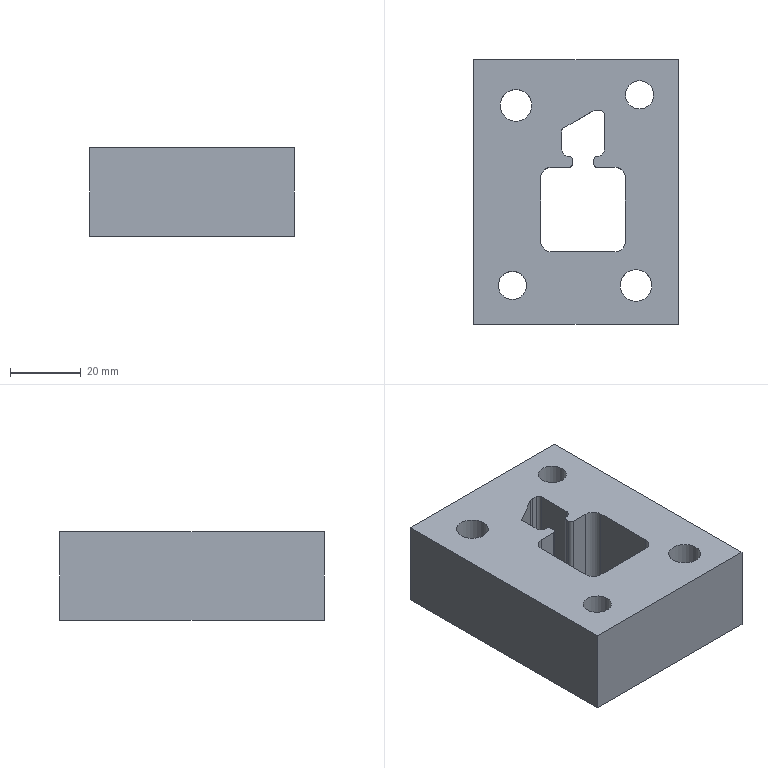Part | STEP file | gslz 2016.10.28-10_id50_x_t | 1 solid | 42 faces | box 58 x 75 x 25 mm | volume 81544 mm3 | plane 21 | cylinder 21 | commonest cylinder face diameters 2 x5 6 x4 4 x3 8 x2 9 x2 10 x2